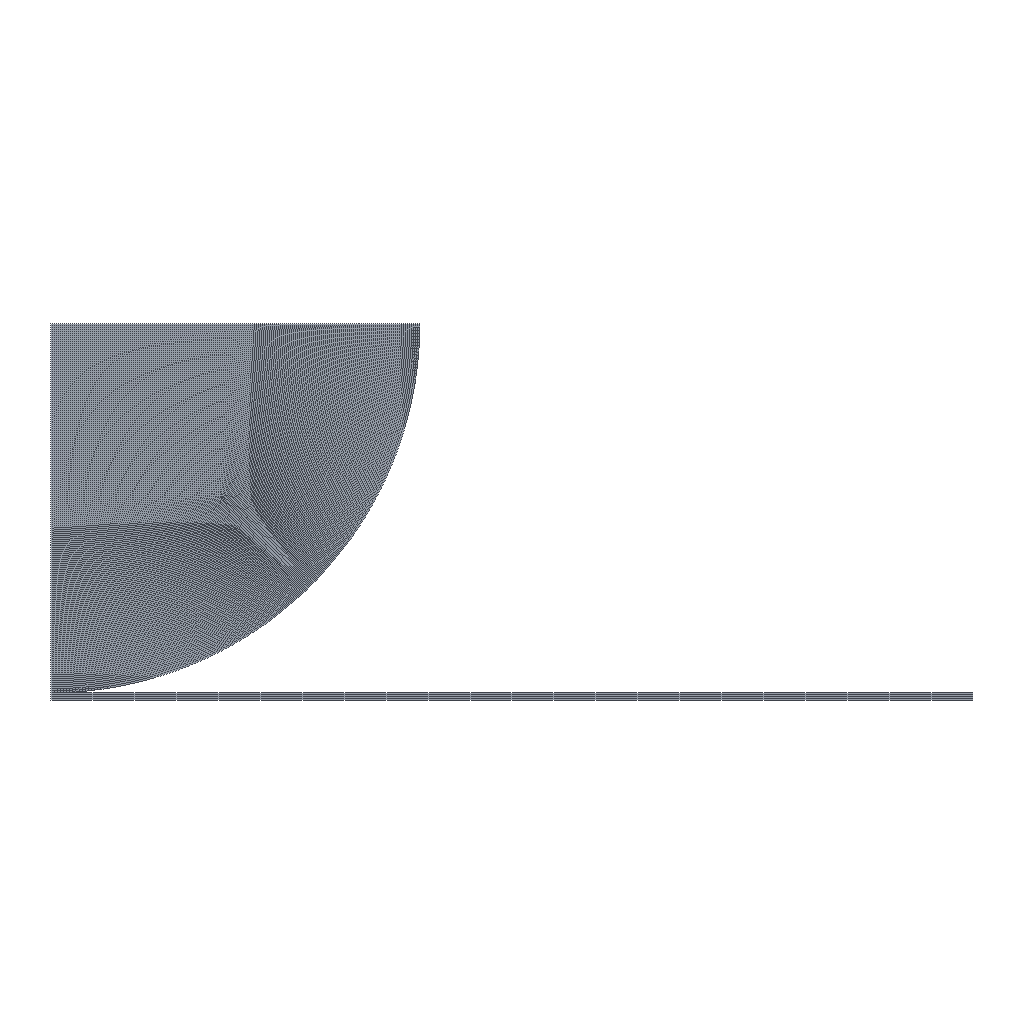Simulation study | abaqus
Set-up summary:
category,name,step,type,value,unit,region
solver,abaqus,,Abaqus/CAE 2024
units,mm-N-s-tonne (MPa),,inferred,E=200000 density=
analysis,Step-1,,static,nlgeom=True; time_period=1
mesh,nodes,,,27546
mesh,elements,,,26961
element_type,CAX4R,,,26961
material,Material-2,,E,200000
material,Material-2,,nu,0.3
material,steel,,E,200000
material,steel,,nu,0.3
material,steel,,yield,355.6
material,steel,,behaviors,plastic
section,steel,,solid section,,,Set-1
section,steel,,solid section,,,Set-1
bc,Fixed-disk,initial,fixed,"[dofs=rz,x,y n=3]",,Set-3
bc,Symm,initial,zsymm,[dofs=ZSYMM],,Set-4
bc,BC-3,Step-1,fixed,"[dofs=rz,x n=2]",,Set-6
bc,BC-3,Step-1,displacement,-0.4 [dofs=y],,Set-6
contact,ball-disk,initial,contact pair surface to surface,interaction=IntProp-1; friction=0; behavior=hard,,s_Surf-1 / m_Surf-1
constraint,rigid body,,,1
Abaqus input file, long lists of numbers shortened:
*Heading
** Job name: deck Model name: Model-1
** Generated by: Abaqus/CAE 2024
*Preprint, echo=NO, model=NO, history=NO, contact=NO
**
** PARTS
**
*Part, name=ball
*Node
      1,   7.041,   2.899
      2,          10.,          10.
** (26038 more lines like these left out)
*Element, type=CAX4R
    1,     1,     8,   833,   375
    2,     8,     9,   834,   833
** (25759 more lines like these left out)
*Nset, nset=Set-1, generate
     1,  26040,      1
*Elset, elset=Set-1, generate
     1,  25761,      1
*Nset, nset=Set-4, generate
     1,  26040,      1
*Elset, elset=Set-4, generate
     1,  25761,      1
** Section: Section-1
*Solid Section, elset=Set-1, material=steel
,
*End Part
**
*Part, name=disk
*Node
      1,          25.,           0.
      2,    24.917,           0.
** (1503 more lines like these left out)
*Element, type=CAX4R
   1,    1,    2,  303,  302
   2,    2,    3,  304,  303
** (1198 more lines like these left out)
*Nset, nset=Set-1, generate
    1,  1505,     1
*Elset, elset=Set-1, generate
    1,  1200,     1
*Nset, nset=Set-5, generate
    1,  1505,     1
*Elset, elset=Set-5, generate
    1,  1200,     1
** Section: Section-1
*Solid Section, elset=Set-1, material=steel
,
*End Part
**
**
** ASSEMBLY
**
*Assembly, name=Assembly
**
*Instance, name=ball-1, part=ball
*End Instance
**
*Instance, name=disk-1, part=disk
*End Instance
**
*Node
      1,           0.,           0.,           0.
*Nset, nset=Set-3, instance=disk-1, generate
    1,  1205,   301
*Elset, elset=Set-3, instance=disk-1, generate
   1,  901,  300
*Nset, nset=Set-4, instance=ball-1
   5,   6,   7, 467, 468, 469, 470, 471, 472, 473, 474, 475, 476, 477, 478, 479
 480, 481, 482, 483, 484, 485, 486, 487, 488, 489, 490, 491, 492, 493, 494, 495
** (10 more lines like these left out)
*Nset, nset=Set-4, instance=disk-1, generate
  301,  1505,   301
*Elset, elset=Set-4, instance=ball-1
  8741,  8833,  8925,  9017,  9109,  9201,  9293,  9385,  9477,  9569,  9661,  9753,  9845,  9937, 10029, 10121
 10213, 10305, 10397, 10489, 10581, 10673, 10765, 10857, 10949, 11041, 11133, 11225, 11317, 11409, 11501, 11593
** (10 more lines like these left out)
*Elset, elset=Set-4, instance=disk-1, generate
  300,  1200,   300
*Nset, nset=Set-5, instance=ball-1
 5,
*Nset, nset=Set-6, instance=ball-1, generate
     1,  26040,      1
*Elset, elset=Set-6, instance=ball-1, generate
     1,  25761,      1
*Nset, nset=b_Set-1, instance=ball-1, generate
     1,  26040,      1
*Elset, elset=b_Set-1, instance=ball-1, generate
     1,  25761,      1
*Nset, nset=_PickedSet8, internal
 1,
*Elset, elset=_m_Surf-1_S1, internal, instance=ball-1, generate
  1,  93,   1
*Elset, elset=_m_Surf-1_S2, internal, instance=ball-1, generate
 17298,  25761,     93
*Surface, type=ELEMENT, name=m_Surf-1
_m_Surf-1_S1, S1
_m_Surf-1_S2, S2
*Elset, elset=_s_Surf-1_S1, internal, instance=disk-1, generate
   1,  300,    1
*Surface, type=ELEMENT, name=s_Surf-1
_s_Surf-1_S1, S1
** Constraint: Constraint-1
*Rigid Body, ref node=_PickedSet8, elset=b_Set-1
*End Assembly
**
** MATERIALS
**
*Material, name=Material-2
*Elastic
200000., 0.3
*Material, name=steel
*Elastic
200000., 0.3
*Plastic
   355.6,       0.
  356.42, 0.002295
  357.13, 0.004281
  357.84, 0.006264
  358.55, 0.008243
  359.26, 0.01022
  359.97, 0.01219
  360.68, 0.01416
  361.39, 0.01612
   362.1, 0.01808
  371.88, 0.01999
 381.696, 0.0219
 391.547, 0.0238
 401.434, 0.0257
 411.356,   0.0276
 421.314, 0.0304
 434.218, 0.03602
 446.324,  0.04125
**
** INTERACTION PROPERTIES
**
*Surface Interaction, name=IntProp-1
1.,
*Friction
0.,
*Surface Behavior, pressure-overclosure=HARD
**
** BOUNDARY CONDITIONS
**
** Name: Fixed-disk Type: Displacement/Rotation
*Boundary
Set-3, 1, 1
Set-3, 2, 2
Set-3, 6, 6
** Name: Symm Type: Symmetry/Antisymmetry/Encastre
*Boundary
Set-4, ZSYMM
**
** INTERACTIONS
**
** Interaction: ball-disk
*Contact Pair, interaction=IntProp-1, type=SURFACE TO SURFACE
s_Surf-1, m_Surf-1
** ----------------------------------------------------------------
**
** STEP: Step-1
**
*Step, name=Step-1, nlgeom=YES, inc=10000
*Static
0.1, 1., 1e-05, 1.
**
** BOUNDARY CONDITIONS
**
** Name: BC-3 Type: Displacement/Rotation
*Boundary
Set-6, 1, 1
Set-6, 2, 2, -0.4
Set-6, 6, 6
**
** OUTPUT REQUESTS
**
*Restart, write, frequency=0
**
** FIELD OUTPUT: F-Output-1
**
*Output, field
*Node Output
U,
*Element Output, directions=YES
E, EE, PE, S, PEEQ
**
** HISTORY OUTPUT: H-Output-1
**
*Output, history, variable=PRESELECT
*End Step
Results summary:
result,odb.job_status,,,JOB_STATUS_COMPLETED_SUCCESSFULLY,"consistent, unstated (Abaqus has no unit system)"
result,steps[0].procedure,Step-1,,*STATIC,"consistent, unstated (Abaqus has no unit system)"
result,steps[0].time_period,Step-1,,1,"consistent, unstated (Abaqus has no unit system)"
result,steps[0].n_frames,Step-1,,13,"consistent, unstated (Abaqus has no unit system)"
result,steps[0].last_frame.id,Step-1,,12,"consistent, unstated (Abaqus has no unit system)"
result,steps[0].last_frame.value,Step-1,,1,"consistent, unstated (Abaqus has no unit system)"
result,steps[0].last_frame.description,Step-1,,Increment     12: Step Time =    1.000,"consistent, unstated (Abaqus has no unit system)"
result,steps[0].completed,Step-1,,True,"consistent, unstated (Abaqus has no unit system)"
result,steps[0].max_U_magnitude,Step-1,,0.4,"consistent, unstated (Abaqus has no unit system)"
result,steps[0].max_S_mises,Step-1,,357.641,"consistent, unstated (Abaqus has no unit system)"
result,steps[0].diagnostic.n_increments,Step-1,,12,"consistent, unstated (Abaqus has no unit system)"
result,steps[1].procedure,Step-1,,*STATIC,"consistent, unstated (Abaqus has no unit system)"
result,steps[1].time_period,Step-1,,1,"consistent, unstated (Abaqus has no unit system)"
result,steps[1].n_frames,Step-1,,7,"consistent, unstated (Abaqus has no unit system)"
result,steps[1].last_frame.id,Step-1,,6,"consistent, unstated (Abaqus has no unit system)"
result,steps[1].last_frame.value,Step-1,,1,"consistent, unstated (Abaqus has no unit system)"
result,steps[1].last_frame.description,Step-1,,Increment      6: Step Time =    1.000,"consistent, unstated (Abaqus has no unit system)"
result,steps[1].completed,Step-1,,True,"consistent, unstated (Abaqus has no unit system)"
result,steps[1].max_U_magnitude,Step-1,,0.4,"consistent, unstated (Abaqus has no unit system)"
result,steps[1].max_S_mises,Step-1,,655.937,"consistent, unstated (Abaqus has no unit system)"
result,steps[1].RF_sum[1],Step-1,,515.426,"consistent, unstated (Abaqus has no unit system)"
result,steps[1].RF_sum[2],Step-1,,0.001337,"consistent, unstated (Abaqus has no unit system)"
result,steps[1].diagnostic.n_increments,Step-1,,6,"consistent, unstated (Abaqus has no unit system)"